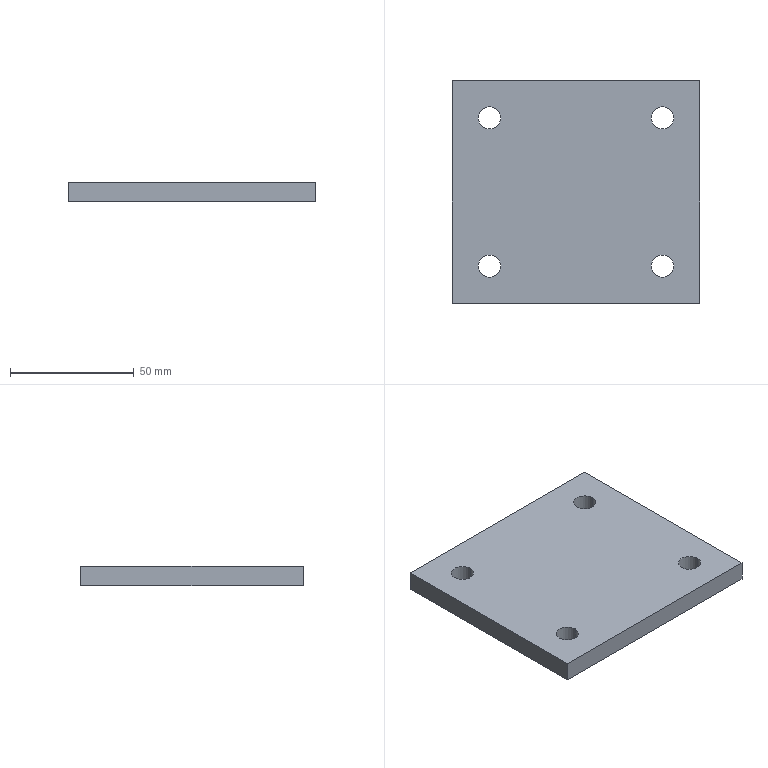Part | SolidWorks | features Extrusion 1, ICE 1 | 1 solid | 14 faces | box 100 x 90 x 8 mm | volume 69964 mm3 | cylinder 8 | plane 6 | commonest cylinder face diameters 9 x8
STEP:
#1=CARTESIAN_POINT('',(30.5,-30.,-4.));
#2=VERTEX_POINT('',#1);
#3=CARTESIAN_POINT('',(39.5,-30.,-4.));
#4=VERTEX_POINT('',#3);
#5=CARTESIAN_POINT('',(35.,-30.,-4.));
#6=DIRECTION('',(0.,0.,1.));
#7=DIRECTION('',(1.,0.,0.));
#8=AXIS2_PLACEMENT_3D('',#5,#6,#7);
#9=CIRCLE('',#8,4.5);
#10=EDGE_CURVE('',#2,#4,#9,.T.);
#11=ORIENTED_EDGE('',*,*,#10,.F.);
#12=CARTESIAN_POINT('',(30.5,-30.,4.));
#13=VERTEX_POINT('',#12);
#14=CARTESIAN_POINT('',(30.5,-30.,-14.));
#15=DIRECTION('',(0.,0.,1.));
#16=VECTOR('',#15,1000.);
#17=LINE('',#14,#16);
#18=EDGE_CURVE('',#2,#13,#17,.T.);
#19=ORIENTED_EDGE('',*,*,#18,.T.);
#20=CARTESIAN_POINT('',(39.5,-30.,4.));
#21=VERTEX_POINT('',#20);
#22=CARTESIAN_POINT('',(35.,-30.,4.));
#23=DIRECTION('',(0.,0.,1.));
#24=DIRECTION('',(1.,0.,0.));
#25=AXIS2_PLACEMENT_3D('',#22,#23,#24);
#26=CIRCLE('',#25,4.5);
#27=EDGE_CURVE('',#13,#21,#26,.T.);
#28=ORIENTED_EDGE('',*,*,#27,.T.);
#29=CARTESIAN_POINT('',(39.5,-30.,-14.));
#30=DIRECTION('',(0.,0.,1.));
#31=VECTOR('',#30,1000.);
#32=LINE('',#29,#31);
#33=EDGE_CURVE('',#4,#21,#32,.T.);
#34=ORIENTED_EDGE('',*,*,#33,.F.);
#35=EDGE_LOOP('',(#11,#19,#28,#34));
#36=FACE_OUTER_BOUND('',#35,.T.);
#37=CARTESIAN_POINT('',(35.,-30.,-14.));
#38=DIRECTION('',(0.,0.,1.));
#39=DIRECTION('',(1.,0.,0.));
#40=AXIS2_PLACEMENT_3D('',#37,#38,#39);
#41=CYLINDRICAL_SURFACE('',#40,4.5);
#42=ADVANCED_FACE('',(#36),#41,.F.);
#43=CARTESIAN_POINT('',(-39.5,30.,-4.));
#44=VERTEX_POINT('',#43);
#45=CARTESIAN_POINT('',(-30.5,30.,-4.));
#46=VERTEX_POINT('',#45);
#47=CARTESIAN_POINT('',(-35.,30.,-4.));
#48=DIRECTION('',(0.,0.,1.));
#49=DIRECTION('',(1.,0.,0.));
#50=AXIS2_PLACEMENT_3D('',#47,#48,#49);
#51=CIRCLE('',#50,4.5);
#52=EDGE_CURVE('',#44,#46,#51,.T.);
#53=ORIENTED_EDGE('',*,*,#52,.F.);
#54=CARTESIAN_POINT('',(-39.5,30.,4.));
#55=VERTEX_POINT('',#54);
#56=CARTESIAN_POINT('',(-39.5,30.,-14.));
#57=DIRECTION('',(0.,0.,1.));
#58=VECTOR('',#57,1000.);
#59=LINE('',#56,#58);
#60=EDGE_CURVE('',#44,#55,#59,.T.);
#61=ORIENTED_EDGE('',*,*,#60,.T.);
#62=CARTESIAN_POINT('',(-30.5,30.,4.));
#63=VERTEX_POINT('',#62);
#64=CARTESIAN_POINT('',(-35.,30.,4.));
#65=DIRECTION('',(0.,0.,1.));
#66=DIRECTION('',(1.,0.,0.));
#67=AXIS2_PLACEMENT_3D('',#64,#65,#66);
#68=CIRCLE('',#67,4.5);
#69=EDGE_CURVE('',#55,#63,#68,.T.);
#70=ORIENTED_EDGE('',*,*,#69,.T.);
#71=CARTESIAN_POINT('',(-30.5,30.,-14.));
#72=DIRECTION('',(0.,0.,1.));
#73=VECTOR('',#72,1000.);
#74=LINE('',#71,#73);
#75=EDGE_CURVE('',#46,#63,#74,.T.);
#76=ORIENTED_EDGE('',*,*,#75,.F.);
#77=EDGE_LOOP('',(#53,#61,#70,#76));
#78=FACE_OUTER_BOUND('',#77,.T.);
#79=CARTESIAN_POINT('',(-35.,30.,-14.));
#80=DIRECTION('',(0.,0.,1.));
#81=DIRECTION('',(1.,0.,0.));
#82=AXIS2_PLACEMENT_3D('',#79,#80,#81);
#83=CYLINDRICAL_SURFACE('',#82,4.5);
#84=ADVANCED_FACE('',(#78),#83,.F.);
#85=CARTESIAN_POINT('',(30.5,30.,-4.));
#86=VERTEX_POINT('',#85);
#87=CARTESIAN_POINT('',(39.5,30.,-4.));
#88=VERTEX_POINT('',#87);
#89=CARTESIAN_POINT('',(35.,30.,-4.));
#90=DIRECTION('',(0.,0.,1.));
#91=DIRECTION('',(1.,0.,0.));
#92=AXIS2_PLACEMENT_3D('',#89,#90,#91);
#93=CIRCLE('',#92,4.5);
#94=EDGE_CURVE('',#86,#88,#93,.T.);
#95=ORIENTED_EDGE('',*,*,#94,.F.);
#96=CARTESIAN_POINT('',(30.5,30.,4.));
#97=VERTEX_POINT('',#96);
#98=CARTESIAN_POINT('',(30.5,30.,-14.));
#99=DIRECTION('',(0.,0.,1.));
#100=VECTOR('',#99,1000.);
#101=LINE('',#98,#100);
#102=EDGE_CURVE('',#86,#97,#101,.T.);
#103=ORIENTED_EDGE('',*,*,#102,.T.);
#104=CARTESIAN_POINT('',(39.5,30.,4.));
#105=VERTEX_POINT('',#104);
#106=CARTESIAN_POINT('',(35.,30.,4.));
#107=DIRECTION('',(0.,0.,1.));
#108=DIRECTION('',(1.,0.,0.));
#109=AXIS2_PLACEMENT_3D('',#106,#107,#108);
#110=CIRCLE('',#109,4.5);
#111=EDGE_CURVE('',#97,#105,#110,.T.);
#112=ORIENTED_EDGE('',*,*,#111,.T.);
#113=CARTESIAN_POINT('',(39.5,30.,-14.));
#114=DIRECTION('',(0.,0.,1.));
#115=VECTOR('',#114,1000.);
#116=LINE('',#113,#115);
#117=EDGE_CURVE('',#88,#105,#116,.T.);
#118=ORIENTED_EDGE('',*,*,#117,.F.);
#119=EDGE_LOOP('',(#95,#103,#112,#118));
#120=FACE_OUTER_BOUND('',#119,.T.);
#121=CARTESIAN_POINT('',(35.,30.,-14.));
#122=DIRECTION('',(0.,0.,1.));
#123=DIRECTION('',(1.,0.,0.));
#124=AXIS2_PLACEMENT_3D('',#121,#122,#123);
#125=CYLINDRICAL_SURFACE('',#124,4.5);
#126=ADVANCED_FACE('',(#120),#125,.F.);
#127=CARTESIAN_POINT('',(-39.5,-30.,-4.));
#128=VERTEX_POINT('',#127);
#129=CARTESIAN_POINT('',(-30.5,-30.,-4.));
#130=VERTEX_POINT('',#129);
#131=CARTESIAN_POINT('',(-35.,-30.,-4.));
#132=DIRECTION('',(0.,0.,1.));
#133=DIRECTION('',(1.,0.,0.));
#134=AXIS2_PLACEMENT_3D('',#131,#132,#133);
#135=CIRCLE('',#134,4.5);
#136=EDGE_CURVE('',#128,#130,#135,.T.);
#137=ORIENTED_EDGE('',*,*,#136,.F.);
#138=CARTESIAN_POINT('',(-39.5,-30.,4.));
#139=VERTEX_POINT('',#138);
#140=CARTESIAN_POINT('',(-39.5,-30.,-14.));
#141=DIRECTION('',(0.,0.,1.));
#142=VECTOR('',#141,1000.);
#143=LINE('',#140,#142);
#144=EDGE_CURVE('',#128,#139,#143,.T.);
#145=ORIENTED_EDGE('',*,*,#144,.T.);
#146=CARTESIAN_POINT('',(-30.5,-30.,4.));
#147=VERTEX_POINT('',#146);
#148=CARTESIAN_POINT('',(-35.,-30.,4.));
#149=DIRECTION('',(0.,0.,1.));
#150=DIRECTION('',(1.,0.,0.));
#151=AXIS2_PLACEMENT_3D('',#148,#149,#150);
#152=CIRCLE('',#151,4.5);
#153=EDGE_CURVE('',#139,#147,#152,.T.);
#154=ORIENTED_EDGE('',*,*,#153,.T.);
#155=CARTESIAN_POINT('',(-30.5,-30.,-14.));
#156=DIRECTION('',(0.,0.,1.));
#157=VECTOR('',#156,1000.);
#158=LINE('',#155,#157);
#159=EDGE_CURVE('',#130,#147,#158,.T.);
#160=ORIENTED_EDGE('',*,*,#159,.F.);
#161=EDGE_LOOP('',(#137,#145,#154,#160));
#162=FACE_OUTER_BOUND('',#161,.T.);
#163=CARTESIAN_POINT('',(-35.,-30.,-14.));
#164=DIRECTION('',(0.,0.,1.));
#165=DIRECTION('',(1.,0.,0.));
#166=AXIS2_PLACEMENT_3D('',#163,#164,#165);
#167=CYLINDRICAL_SURFACE('',#166,4.5);
#168=ADVANCED_FACE('',(#162),#167,.F.);
#169=CARTESIAN_POINT('',(-50.,45.,4.));
#170=VERTEX_POINT('',#169);
#171=CARTESIAN_POINT('',(-50.,-45.,4.));
#172=VERTEX_POINT('',#171);
#173=CARTESIAN_POINT('',(-50.,45.,4.));
#174=DIRECTION('',(0.,-1.,0.));
#175=VECTOR('',#174,1000.);
#176=LINE('',#173,#175);
#177=EDGE_CURVE('',#170,#172,#176,.T.);
#178=ORIENTED_EDGE('',*,*,#177,.F.);
#179=CARTESIAN_POINT('',(-50.,45.,-4.));
#180=VERTEX_POINT('',#179);
#181=CARTESIAN_POINT('',(-50.,45.,-4.));
#182=DIRECTION('',(0.,0.,1.));
#183=VECTOR('',#182,1000.);
#184=LINE('',#181,#183);
#185=EDGE_CURVE('',#180,#170,#184,.T.);
#186=ORIENTED_EDGE('',*,*,#185,.F.);
#187=CARTESIAN_POINT('',(-50.,-45.,-4.));
#188=VERTEX_POINT('',#187);
#189=CARTESIAN_POINT('',(-50.,45.,-4.));
#190=DIRECTION('',(0.,-1.,0.));
#191=VECTOR('',#190,1000.);
#192=LINE('',#189,#191);
#193=EDGE_CURVE('',#180,#188,#192,.T.);
#194=ORIENTED_EDGE('',*,*,#193,.T.);
#195=CARTESIAN_POINT('',(-50.,-45.,-4.));
#196=DIRECTION('',(0.,0.,1.));
#197=VECTOR('',#196,1000.);
#198=LINE('',#195,#197);
#199=EDGE_CURVE('',#188,#172,#198,.T.);
#200=ORIENTED_EDGE('',*,*,#199,.T.);
#201=EDGE_LOOP('',(#178,#186,#194,#200));
#202=FACE_OUTER_BOUND('',#201,.T.);
#203=CARTESIAN_POINT('',(-50.,45.,-4.));
#204=DIRECTION('',(-1.,0.,0.));
#205=DIRECTION('',(0.,0.,1.));
#206=AXIS2_PLACEMENT_3D('',#203,#204,#205);
#207=PLANE('',#206);
#208=ADVANCED_FACE('',(#202),#207,.T.);
#209=CARTESIAN_POINT('',(50.,45.,4.));
#210=VERTEX_POINT('',#209);
#211=CARTESIAN_POINT('',(50.,45.,4.));
#212=DIRECTION('',(-1.,0.,0.));
#213=VECTOR('',#212,1000.);
#214=LINE('',#211,#213);
#215=EDGE_CURVE('',#210,#170,#214,.T.);
#216=ORIENTED_EDGE('',*,*,#215,.F.);
#217=CARTESIAN_POINT('',(50.,45.,-4.));
#218=VERTEX_POINT('',#217);
#219=CARTESIAN_POINT('',(50.,45.,-4.));
#220=DIRECTION('',(0.,0.,1.));
#221=VECTOR('',#220,1000.);
#222=LINE('',#219,#221);
#223=EDGE_CURVE('',#218,#210,#222,.T.);
#224=ORIENTED_EDGE('',*,*,#223,.F.);
#225=CARTESIAN_POINT('',(50.,45.,-4.));
#226=DIRECTION('',(-1.,0.,0.));
#227=VECTOR('',#226,1000.);
#228=LINE('',#225,#227);
#229=EDGE_CURVE('',#218,#180,#228,.T.);
#230=ORIENTED_EDGE('',*,*,#229,.T.);
#231=ORIENTED_EDGE('',*,*,#185,.T.);
#232=EDGE_LOOP('',(#216,#224,#230,#231));
#233=FACE_OUTER_BOUND('',#232,.T.);
#234=CARTESIAN_POINT('',(50.,45.,-4.));
#235=DIRECTION('',(0.,1.,0.));
#236=DIRECTION('',(0.,0.,1.));
#237=AXIS2_PLACEMENT_3D('',#234,#235,#236);
#238=PLANE('',#237);
#239=ADVANCED_FACE('',(#233),#238,.T.);
#240=CARTESIAN_POINT('',(50.,-45.,4.));
#241=VERTEX_POINT('',#240);
#242=CARTESIAN_POINT('',(50.,-45.,4.));
#243=DIRECTION('',(0.,1.,0.));
#244=VECTOR('',#243,1000.);
#245=LINE('',#242,#244);
#246=EDGE_CURVE('',#241,#210,#245,.T.);
#247=ORIENTED_EDGE('',*,*,#246,.F.);
#248=CARTESIAN_POINT('',(50.,-45.,-4.));
#249=VERTEX_POINT('',#248);
#250=CARTESIAN_POINT('',(50.,-45.,-4.));
#251=DIRECTION('',(0.,0.,1.));
#252=VECTOR('',#251,1000.);
#253=LINE('',#250,#252);
#254=EDGE_CURVE('',#249,#241,#253,.T.);
#255=ORIENTED_EDGE('',*,*,#254,.F.);
#256=CARTESIAN_POINT('',(50.,-45.,-4.));
#257=DIRECTION('',(0.,1.,0.));
#258=VECTOR('',#257,1000.);
#259=LINE('',#256,#258);
#260=EDGE_CURVE('',#249,#218,#259,.T.);
#261=ORIENTED_EDGE('',*,*,#260,.T.);
#262=ORIENTED_EDGE('',*,*,#223,.T.);
#263=EDGE_LOOP('',(#247,#255,#261,#262));
#264=FACE_OUTER_BOUND('',#263,.T.);
#265=CARTESIAN_POINT('',(50.,-45.,-4.));
#266=DIRECTION('',(1.,0.,0.));
#267=DIRECTION('',(0.,0.,-1.));
#268=AXIS2_PLACEMENT_3D('',#265,#266,#267);
#269=PLANE('',#268);
#270=ADVANCED_FACE('',(#264),#269,.T.);
#271=CARTESIAN_POINT('',(-50.,-45.,4.));
#272=DIRECTION('',(1.,0.,0.));
#273=VECTOR('',#272,1000.);
#274=LINE('',#271,#273);
#275=EDGE_CURVE('',#172,#241,#274,.T.);
#276=ORIENTED_EDGE('',*,*,#275,.F.);
#277=ORIENTED_EDGE('',*,*,#199,.F.);
#278=CARTESIAN_POINT('',(-50.,-45.,-4.));
#279=DIRECTION('',(1.,0.,0.));
#280=VECTOR('',#279,1000.);
#281=LINE('',#278,#280);
#282=EDGE_CURVE('',#188,#249,#281,.T.);
#283=ORIENTED_EDGE('',*,*,#282,.T.);
#284=ORIENTED_EDGE('',*,*,#254,.T.);
#285=EDGE_LOOP('',(#276,#277,#283,#284));
#286=FACE_OUTER_BOUND('',#285,.T.);
#287=CARTESIAN_POINT('',(-50.,-45.,-4.));
#288=DIRECTION('',(0.,-1.,0.));
#289=DIRECTION('',(0.,0.,-1.));
#290=AXIS2_PLACEMENT_3D('',#287,#288,#289);
#291=PLANE('',#290);
#292=ADVANCED_FACE('',(#286),#291,.T.);
#293=CARTESIAN_POINT('',(35.,-30.,-4.));
#294=DIRECTION('',(0.,0.,1.));
#295=DIRECTION('',(1.,0.,0.));
#296=AXIS2_PLACEMENT_3D('',#293,#294,#295);
#297=CIRCLE('',#296,4.5);
#298=EDGE_CURVE('',#4,#2,#297,.T.);
#299=ORIENTED_EDGE('',*,*,#298,.T.);
#300=ORIENTED_EDGE('',*,*,#10,.T.);
#301=EDGE_LOOP('',(#299,#300));
#302=FACE_BOUND('',#301,.T.);
#303=CARTESIAN_POINT('',(-35.,30.,-4.));
#304=DIRECTION('',(0.,0.,1.));
#305=DIRECTION('',(1.,0.,0.));
#306=AXIS2_PLACEMENT_3D('',#303,#304,#305);
#307=CIRCLE('',#306,4.5);
#308=EDGE_CURVE('',#46,#44,#307,.T.);
#309=ORIENTED_EDGE('',*,*,#308,.T.);
#310=ORIENTED_EDGE('',*,*,#52,.T.);
#311=EDGE_LOOP('',(#309,#310));
#312=FACE_BOUND('',#311,.T.);
#313=CARTESIAN_POINT('',(35.,30.,-4.));
#314=DIRECTION('',(0.,0.,1.));
#315=DIRECTION('',(1.,0.,0.));
#316=AXIS2_PLACEMENT_3D('',#313,#314,#315);
#317=CIRCLE('',#316,4.5);
#318=EDGE_CURVE('',#88,#86,#317,.T.);
#319=ORIENTED_EDGE('',*,*,#318,.T.);
#320=ORIENTED_EDGE('',*,*,#94,.T.);
#321=EDGE_LOOP('',(#319,#320));
#322=FACE_BOUND('',#321,.T.);
#323=CARTESIAN_POINT('',(-35.,-30.,-4.));
#324=DIRECTION('',(0.,0.,1.));
#325=DIRECTION('',(1.,0.,0.));
#326=AXIS2_PLACEMENT_3D('',#323,#324,#325);
#327=CIRCLE('',#326,4.5);
#328=EDGE_CURVE('',#130,#128,#327,.T.);
#329=ORIENTED_EDGE('',*,*,#328,.T.);
#330=ORIENTED_EDGE('',*,*,#136,.T.);
#331=EDGE_LOOP('',(#329,#330));
#332=FACE_BOUND('',#331,.T.);
#333=ORIENTED_EDGE('',*,*,#193,.F.);
#334=ORIENTED_EDGE('',*,*,#229,.F.);
#335=ORIENTED_EDGE('',*,*,#260,.F.);
#336=ORIENTED_EDGE('',*,*,#282,.F.);
#337=EDGE_LOOP('',(#333,#334,#335,#336));
#338=FACE_OUTER_BOUND('',#337,.T.);
#339=CARTESIAN_POINT('',(0.,0.,-4.));
#340=DIRECTION('',(0.,0.,1.));
#341=DIRECTION('',(1.,0.,0.));
#342=AXIS2_PLACEMENT_3D('',#339,#340,#341);
#343=PLANE('',#342);
#344=ADVANCED_FACE('',(#302,#312,#322,#332,#338),#343,.F.);
#345=CARTESIAN_POINT('',(35.,-30.,4.));
#346=DIRECTION('',(0.,0.,1.));
#347=DIRECTION('',(1.,0.,0.));
#348=AXIS2_PLACEMENT_3D('',#345,#346,#347);
#349=CIRCLE('',#348,4.5);
#350=EDGE_CURVE('',#21,#13,#349,.T.);
#351=ORIENTED_EDGE('',*,*,#350,.F.);
#352=ORIENTED_EDGE('',*,*,#27,.F.);
#353=EDGE_LOOP('',(#351,#352));
#354=FACE_BOUND('',#353,.T.);
#355=CARTESIAN_POINT('',(-35.,30.,4.));
#356=DIRECTION('',(0.,0.,1.));
#357=DIRECTION('',(1.,0.,0.));
#358=AXIS2_PLACEMENT_3D('',#355,#356,#357);
#359=CIRCLE('',#358,4.5);
#360=EDGE_CURVE('',#63,#55,#359,.T.);
#361=ORIENTED_EDGE('',*,*,#360,.F.);
#362=ORIENTED_EDGE('',*,*,#69,.F.);
#363=EDGE_LOOP('',(#361,#362));
#364=FACE_BOUND('',#363,.T.);
#365=CARTESIAN_POINT('',(35.,30.,4.));
#366=DIRECTION('',(0.,0.,1.));
#367=DIRECTION('',(1.,0.,0.));
#368=AXIS2_PLACEMENT_3D('',#365,#366,#367);
#369=CIRCLE('',#368,4.5);
#370=EDGE_CURVE('',#105,#97,#369,.T.);
#371=ORIENTED_EDGE('',*,*,#370,.F.);
#372=ORIENTED_EDGE('',*,*,#111,.F.);
#373=EDGE_LOOP('',(#371,#372));
#374=FACE_BOUND('',#373,.T.);
#375=CARTESIAN_POINT('',(-35.,-30.,4.));
#376=DIRECTION('',(0.,0.,1.));
#377=DIRECTION('',(1.,0.,0.));
#378=AXIS2_PLACEMENT_3D('',#375,#376,#377);
#379=CIRCLE('',#378,4.5);
#380=EDGE_CURVE('',#147,#139,#379,.T.);
#381=ORIENTED_EDGE('',*,*,#380,.F.);
#382=ORIENTED_EDGE('',*,*,#153,.F.);
#383=EDGE_LOOP('',(#381,#382));
#384=FACE_BOUND('',#383,.T.);
#385=ORIENTED_EDGE('',*,*,#177,.T.);
#386=ORIENTED_EDGE('',*,*,#275,.T.);
#387=ORIENTED_EDGE('',*,*,#246,.T.);
#388=ORIENTED_EDGE('',*,*,#215,.T.);
#389=EDGE_LOOP('',(#385,#386,#387,#388));
#390=FACE_OUTER_BOUND('',#389,.T.);
#391=CARTESIAN_POINT('',(0.,0.,4.));
#392=DIRECTION('',(0.,0.,1.));
#393=DIRECTION('',(1.,0.,0.));
#394=AXIS2_PLACEMENT_3D('',#391,#392,#393);
#395=PLANE('',#394);
#396=ADVANCED_FACE('',(#354,#364,#374,#384,#390),#395,.T.);
#397=ORIENTED_EDGE('',*,*,#144,.F.);
#398=ORIENTED_EDGE('',*,*,#328,.F.);
#399=ORIENTED_EDGE('',*,*,#159,.T.);
#400=ORIENTED_EDGE('',*,*,#380,.T.);
#401=EDGE_LOOP('',(#397,#398,#399,#400));
#402=FACE_OUTER_BOUND('',#401,.T.);
#403=CARTESIAN_POINT('',(-35.,-30.,-14.));
#404=DIRECTION('',(0.,0.,1.));
#405=DIRECTION('',(1.,0.,0.));
#406=AXIS2_PLACEMENT_3D('',#403,#404,#405);
#407=CYLINDRICAL_SURFACE('',#406,4.5);
#408=ADVANCED_FACE('',(#402),#407,.F.);
#409=ORIENTED_EDGE('',*,*,#102,.F.);
#410=ORIENTED_EDGE('',*,*,#318,.F.);
#411=ORIENTED_EDGE('',*,*,#117,.T.);
#412=ORIENTED_EDGE('',*,*,#370,.T.);
#413=EDGE_LOOP('',(#409,#410,#411,#412));
#414=FACE_OUTER_BOUND('',#413,.T.);
#415=CARTESIAN_POINT('',(35.,30.,-14.));
#416=DIRECTION('',(0.,0.,1.));
#417=DIRECTION('',(1.,0.,0.));
#418=AXIS2_PLACEMENT_3D('',#415,#416,#417);
#419=CYLINDRICAL_SURFACE('',#418,4.5);
#420=ADVANCED_FACE('',(#414),#419,.F.);
#421=ORIENTED_EDGE('',*,*,#60,.F.);
#422=ORIENTED_EDGE('',*,*,#308,.F.);
#423=ORIENTED_EDGE('',*,*,#75,.T.);
#424=ORIENTED_EDGE('',*,*,#360,.T.);
#425=EDGE_LOOP('',(#421,#422,#423,#424));
#426=FACE_OUTER_BOUND('',#425,.T.);
#427=CARTESIAN_POINT('',(-35.,30.,-14.));
#428=DIRECTION('',(0.,0.,1.));
#429=DIRECTION('',(1.,0.,0.));
#430=AXIS2_PLACEMENT_3D('',#427,#428,#429);
#431=CYLINDRICAL_SURFACE('',#430,4.5);
#432=ADVANCED_FACE('',(#426),#431,.F.);
#433=ORIENTED_EDGE('',*,*,#18,.F.);
#434=ORIENTED_EDGE('',*,*,#298,.F.);
#435=ORIENTED_EDGE('',*,*,#33,.T.);
#436=ORIENTED_EDGE('',*,*,#350,.T.);
#437=EDGE_LOOP('',(#433,#434,#435,#436));
#438=FACE_OUTER_BOUND('',#437,.T.);
#439=CARTESIAN_POINT('',(35.,-30.,-14.));
#440=DIRECTION('',(0.,0.,1.));
#441=DIRECTION('',(1.,0.,0.));
#442=AXIS2_PLACEMENT_3D('',#439,#440,#441);
#443=CYLINDRICAL_SURFACE('',#442,4.5);
#444=ADVANCED_FACE('',(#438),#443,.F.);
#445=CLOSED_SHELL('',(#42,#84,#126,#168,#208,#239,#270,#292,#344,#396,#408,#420,#432,#444));
#446=MANIFOLD_SOLID_BREP('',#445);
#447=CARTESIAN_POINT('',(0.,0.,0.));
#448=DIRECTION('',(0.,0.,1.));
#449=DIRECTION('',(1.,0.,0.));
#450=AXIS2_PLACEMENT_3D('',#447,#448,#449);
#451=(LENGTH_UNIT()NAMED_UNIT(*)SI_UNIT(.MILLI.,.METRE.));
#452=UNCERTAINTY_MEASURE_WITH_UNIT(LENGTH_MEASURE(0.00001),#451,'','');
#453=(NAMED_UNIT(*)PLANE_ANGLE_UNIT()SI_UNIT($,.RADIAN.));
#454=(NAMED_UNIT(*)SI_UNIT($,.STERADIAN.)SOLID_ANGLE_UNIT());
#455=(GEOMETRIC_REPRESENTATION_CONTEXT(3)GLOBAL_UNCERTAINTY_ASSIGNED_CONTEXT((#452))GLOBAL_UNIT_ASSIGNED_CONTEXT((#451,#453,#454))REPRESENTATION_CONTEXT('',''));
#456=ADVANCED_BREP_SHAPE_REPRESENTATION('',(#446,#450),#455);